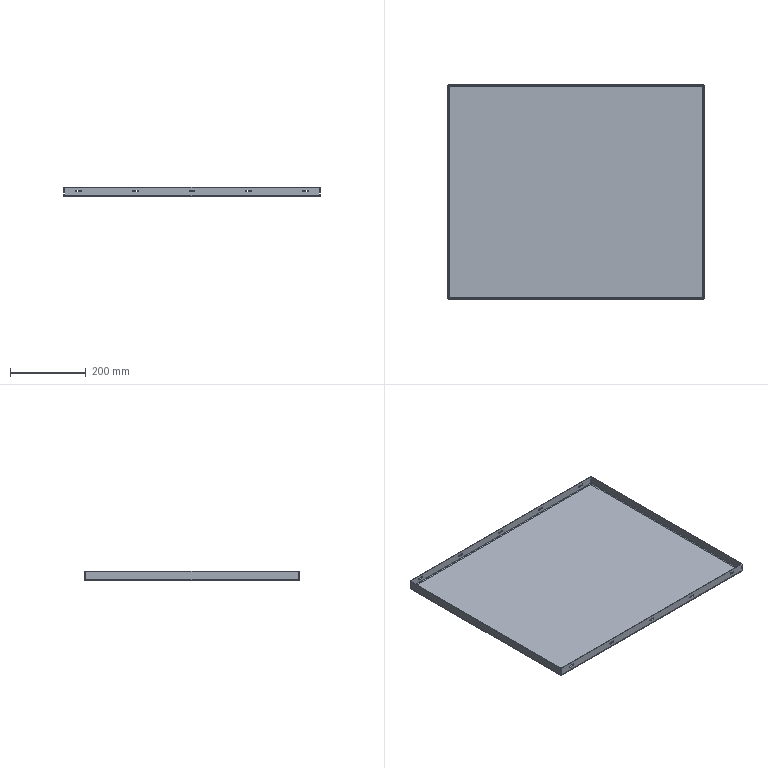Part | SolidWorks | features EdgeFlange 1, FlatPattern 1, ICE 1, SMBaseFlange 1, SheetMetal 1 | 1 solid | 78 faces | box 680 x 568 x 25 mm | volume 878615 mm3 | plane 42 | cylinder 28 | spline 8 | commonest cylinder face diameters 4.5 x20 4 x4 8 x4